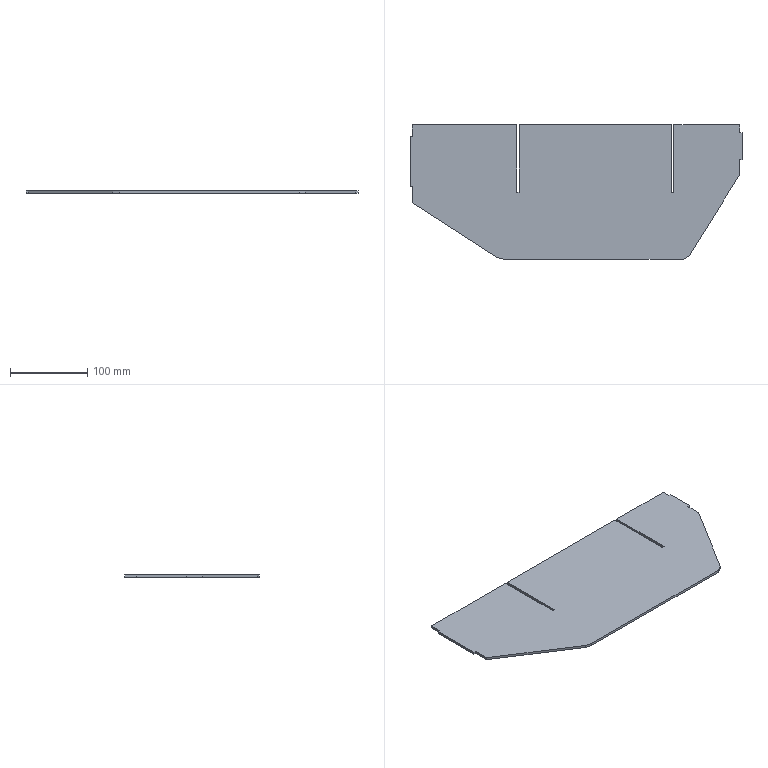Part | SolidWorks | features FlatPattern 1, SMBaseFlange 1, SheetMetal 1 | 1 solid | 26 faces | box 429 x 173.7 x 3.2 mm | volume 209173 mm3 | plane 26
STEP:
#1=CARTESIAN_POINT('',(256.891,49.63,0.));
#2=VERTEX_POINT('',#1);
#3=CARTESIAN_POINT('',(256.891,59.63,0.));
#4=VERTEX_POINT('',#3);
#5=CARTESIAN_POINT('',(256.891,59.63,0.));
#6=DIRECTION('',(0.,1.,0.));
#7=VECTOR('',#6,1000.);
#8=LINE('',#5,#7);
#9=EDGE_CURVE('',#2,#4,#8,.T.);
#10=ORIENTED_EDGE('',*,*,#9,.T.);
#11=CARTESIAN_POINT('',(256.891,59.63,3.2));
#12=VERTEX_POINT('',#11);
#13=CARTESIAN_POINT('',(256.891,59.63,3.2));
#14=DIRECTION('',(0.,0.,-1.));
#15=VECTOR('',#14,1000.);
#16=LINE('',#13,#15);
#17=EDGE_CURVE('',#12,#4,#16,.T.);
#18=ORIENTED_EDGE('',*,*,#17,.F.);
#19=CARTESIAN_POINT('',(256.891,49.63,3.2));
#20=VERTEX_POINT('',#19);
#21=CARTESIAN_POINT('',(256.891,59.63,3.2));
#22=DIRECTION('',(0.,1.,0.));
#23=VECTOR('',#22,1000.);
#24=LINE('',#21,#23);
#25=EDGE_CURVE('',#20,#12,#24,.T.);
#26=ORIENTED_EDGE('',*,*,#25,.F.);
#27=CARTESIAN_POINT('',(256.891,49.63,3.2));
#28=DIRECTION('',(0.,0.,-1.));
#29=VECTOR('',#28,1000.);
#30=LINE('',#27,#29);
#31=EDGE_CURVE('',#20,#2,#30,.T.);
#32=ORIENTED_EDGE('',*,*,#31,.T.);
#33=EDGE_LOOP('',(#10,#18,#26,#32));
#34=FACE_OUTER_BOUND('',#33,.T.);
#35=CARTESIAN_POINT('',(256.891,59.63,3.2));
#36=DIRECTION('',(-1.,0.,0.));
#37=DIRECTION('',(0.,0.,1.));
#38=AXIS2_PLACEMENT_3D('',#35,#36,#37);
#39=PLANE('',#38);
#40=ADVANCED_FACE('',(#34),#39,.F.);
#41=CARTESIAN_POINT('',(171.891,59.63,0.));
#42=VERTEX_POINT('',#41);
#43=CARTESIAN_POINT('',(256.891,59.63,0.));
#44=DIRECTION('',(-1.,0.,0.));
#45=VECTOR('',#44,1000.);
#46=LINE('',#43,#45);
#47=EDGE_CURVE('',#4,#42,#46,.T.);
#48=ORIENTED_EDGE('',*,*,#47,.T.);
#49=CARTESIAN_POINT('',(171.891,59.63,3.2));
#50=VERTEX_POINT('',#49);
#51=CARTESIAN_POINT('',(171.891,59.63,3.2));
#52=DIRECTION('',(0.,0.,-1.));
#53=VECTOR('',#52,1000.);
#54=LINE('',#51,#53);
#55=EDGE_CURVE('',#50,#42,#54,.T.);
#56=ORIENTED_EDGE('',*,*,#55,.F.);
#57=CARTESIAN_POINT('',(256.891,59.63,3.2));
#58=DIRECTION('',(-1.,0.,0.));
#59=VECTOR('',#58,1000.);
#60=LINE('',#57,#59);
#61=EDGE_CURVE('',#12,#50,#60,.T.);
#62=ORIENTED_EDGE('',*,*,#61,.F.);
#63=ORIENTED_EDGE('',*,*,#17,.T.);
#64=EDGE_LOOP('',(#48,#56,#62,#63));
#65=FACE_OUTER_BOUND('',#64,.T.);
#66=CARTESIAN_POINT('',(256.891,59.63,3.2));
#67=DIRECTION('',(0.,-1.,0.));
#68=DIRECTION('',(0.,0.,-1.));
#69=AXIS2_PLACEMENT_3D('',#66,#67,#68);
#70=PLANE('',#69);
#71=ADVANCED_FACE('',(#65),#70,.F.);
#72=CARTESIAN_POINT('',(171.891,-27.37,0.));
#73=VERTEX_POINT('',#72);
#74=CARTESIAN_POINT('',(171.891,-27.37,0.));
#75=DIRECTION('',(0.,-1.,0.));
#76=VECTOR('',#75,1000.);
#77=LINE('',#74,#76);
#78=EDGE_CURVE('',#42,#73,#77,.T.);
#79=ORIENTED_EDGE('',*,*,#78,.T.);
#80=CARTESIAN_POINT('',(171.891,-27.37,3.2));
#81=VERTEX_POINT('',#80);
#82=CARTESIAN_POINT('',(171.891,-27.37,3.2));
#83=DIRECTION('',(0.,0.,-1.));
#84=VECTOR('',#83,1000.);
#85=LINE('',#82,#84);
#86=EDGE_CURVE('',#81,#73,#85,.T.);
#87=ORIENTED_EDGE('',*,*,#86,.F.);
#88=CARTESIAN_POINT('',(171.891,-27.37,3.2));
#89=DIRECTION('',(0.,-1.,0.));
#90=VECTOR('',#89,1000.);
#91=LINE('',#88,#90);
#92=EDGE_CURVE('',#50,#81,#91,.T.);
#93=ORIENTED_EDGE('',*,*,#92,.F.);
#94=ORIENTED_EDGE('',*,*,#55,.T.);
#95=EDGE_LOOP('',(#79,#87,#93,#94));
#96=FACE_OUTER_BOUND('',#95,.T.);
#97=CARTESIAN_POINT('',(171.891,-27.37,3.2));
#98=DIRECTION('',(1.,0.,0.));
#99=DIRECTION('',(0.,1.,0.));
#100=AXIS2_PLACEMENT_3D('',#97,#98,#99);
#101=PLANE('',#100);
#102=ADVANCED_FACE('',(#96),#101,.F.);
#103=CARTESIAN_POINT('',(168.691,-27.37,0.));
#104=VERTEX_POINT('',#103);
#105=CARTESIAN_POINT('',(168.691,-27.37,0.));
#106=DIRECTION('',(-1.,0.,0.));
#107=VECTOR('',#106,1000.);
#108=LINE('',#105,#107);
#109=EDGE_CURVE('',#73,#104,#108,.T.);
#110=ORIENTED_EDGE('',*,*,#109,.T.);
#111=CARTESIAN_POINT('',(168.691,-27.37,3.2));
#112=VERTEX_POINT('',#111);
#113=CARTESIAN_POINT('',(168.691,-27.37,3.2));
#114=DIRECTION('',(0.,0.,-1.));
#115=VECTOR('',#114,1000.);
#116=LINE('',#113,#115);
#117=EDGE_CURVE('',#112,#104,#116,.T.);
#118=ORIENTED_EDGE('',*,*,#117,.F.);
#119=CARTESIAN_POINT('',(168.691,-27.37,3.2));
#120=DIRECTION('',(-1.,0.,0.));
#121=VECTOR('',#120,1000.);
#122=LINE('',#119,#121);
#123=EDGE_CURVE('',#81,#112,#122,.T.);
#124=ORIENTED_EDGE('',*,*,#123,.F.);
#125=ORIENTED_EDGE('',*,*,#86,.T.);
#126=EDGE_LOOP('',(#110,#118,#124,#125));
#127=FACE_OUTER_BOUND('',#126,.T.);
#128=CARTESIAN_POINT('',(168.691,-27.37,3.2));
#129=DIRECTION('',(0.,-1.,0.));
#130=DIRECTION('',(0.,0.,-1.));
#131=AXIS2_PLACEMENT_3D('',#128,#129,#130);
#132=PLANE('',#131);
#133=ADVANCED_FACE('',(#127),#132,.F.);
#134=CARTESIAN_POINT('',(168.691,59.63,0.));
#135=VERTEX_POINT('',#134);
#136=CARTESIAN_POINT('',(168.691,59.63,0.));
#137=DIRECTION('',(0.,1.,0.));
#138=VECTOR('',#137,1000.);
#139=LINE('',#136,#138);
#140=EDGE_CURVE('',#104,#135,#139,.T.);
#141=ORIENTED_EDGE('',*,*,#140,.T.);
#142=CARTESIAN_POINT('',(168.691,59.63,3.2));
#143=VERTEX_POINT('',#142);
#144=CARTESIAN_POINT('',(168.691,59.63,3.2));
#145=DIRECTION('',(0.,0.,-1.));
#146=VECTOR('',#145,1000.);
#147=LINE('',#144,#146);
#148=EDGE_CURVE('',#143,#135,#147,.T.);
#149=ORIENTED_EDGE('',*,*,#148,.F.);
#150=CARTESIAN_POINT('',(168.691,59.63,3.2));
#151=DIRECTION('',(0.,1.,0.));
#152=VECTOR('',#151,1000.);
#153=LINE('',#150,#152);
#154=EDGE_CURVE('',#112,#143,#153,.T.);
#155=ORIENTED_EDGE('',*,*,#154,.F.);
#156=ORIENTED_EDGE('',*,*,#117,.T.);
#157=EDGE_LOOP('',(#141,#149,#155,#156));
#158=FACE_OUTER_BOUND('',#157,.T.);
#159=CARTESIAN_POINT('',(168.691,59.63,3.2));
#160=DIRECTION('',(-1.,0.,0.));
#161=DIRECTION('',(0.,-1.,0.));
#162=AXIS2_PLACEMENT_3D('',#159,#160,#161);
#163=PLANE('',#162);
#164=ADVANCED_FACE('',(#158),#163,.F.);
#165=CARTESIAN_POINT('',(-28.109,59.63,0.));
#166=VERTEX_POINT('',#165);
#167=CARTESIAN_POINT('',(168.691,59.63,0.));
#168=DIRECTION('',(-1.,0.,0.));
#169=VECTOR('',#168,1000.);
#170=LINE('',#167,#169);
#171=EDGE_CURVE('',#135,#166,#170,.T.);
#172=ORIENTED_EDGE('',*,*,#171,.T.);
#173=CARTESIAN_POINT('',(-28.109,59.63,3.2));
#174=VERTEX_POINT('',#173);
#175=CARTESIAN_POINT('',(-28.109,59.63,3.2));
#176=DIRECTION('',(0.,0.,-1.));
#177=VECTOR('',#176,1000.);
#178=LINE('',#175,#177);
#179=EDGE_CURVE('',#174,#166,#178,.T.);
#180=ORIENTED_EDGE('',*,*,#179,.F.);
#181=CARTESIAN_POINT('',(168.691,59.63,3.2));
#182=DIRECTION('',(-1.,0.,0.));
#183=VECTOR('',#182,1000.);
#184=LINE('',#181,#183);
#185=EDGE_CURVE('',#143,#174,#184,.T.);
#186=ORIENTED_EDGE('',*,*,#185,.F.);
#187=ORIENTED_EDGE('',*,*,#148,.T.);
#188=EDGE_LOOP('',(#172,#180,#186,#187));
#189=FACE_OUTER_BOUND('',#188,.T.);
#190=CARTESIAN_POINT('',(168.691,59.63,3.2));
#191=DIRECTION('',(0.,-1.,0.));
#192=DIRECTION('',(0.,0.,-1.));
#193=AXIS2_PLACEMENT_3D('',#190,#191,#192);
#194=PLANE('',#193);
#195=ADVANCED_FACE('',(#189),#194,.F.);
#196=CARTESIAN_POINT('',(-28.109,-27.37,0.));
#197=VERTEX_POINT('',#196);
#198=CARTESIAN_POINT('',(-28.109,-27.37,0.));
#199=DIRECTION('',(0.,-1.,0.));
#200=VECTOR('',#199,1000.);
#201=LINE('',#198,#200);
#202=EDGE_CURVE('',#166,#197,#201,.T.);
#203=ORIENTED_EDGE('',*,*,#202,.T.);
#204=CARTESIAN_POINT('',(-28.109,-27.37,3.2));
#205=VERTEX_POINT('',#204);
#206=CARTESIAN_POINT('',(-28.109,-27.37,3.2));
#207=DIRECTION('',(0.,0.,-1.));
#208=VECTOR('',#207,1000.);
#209=LINE('',#206,#208);
#210=EDGE_CURVE('',#205,#197,#209,.T.);
#211=ORIENTED_EDGE('',*,*,#210,.F.);
#212=CARTESIAN_POINT('',(-28.109,-27.37,3.2));
#213=DIRECTION('',(0.,-1.,0.));
#214=VECTOR('',#213,1000.);
#215=LINE('',#212,#214);
#216=EDGE_CURVE('',#174,#205,#215,.T.);
#217=ORIENTED_EDGE('',*,*,#216,.F.);
#218=ORIENTED_EDGE('',*,*,#179,.T.);
#219=EDGE_LOOP('',(#203,#211,#217,#218));
#220=FACE_OUTER_BOUND('',#219,.T.);
#221=CARTESIAN_POINT('',(-28.109,-27.37,3.2));
#222=DIRECTION('',(1.,0.,0.));
#223=DIRECTION('',(0.,1.,0.));
#224=AXIS2_PLACEMENT_3D('',#221,#222,#223);
#225=PLANE('',#224);
#226=ADVANCED_FACE('',(#220),#225,.F.);
#227=CARTESIAN_POINT('',(-31.309,-27.37,0.));
#228=VERTEX_POINT('',#227);
#229=CARTESIAN_POINT('',(-31.309,-27.37,0.));
#230=DIRECTION('',(-1.,0.,0.));
#231=VECTOR('',#230,1000.);
#232=LINE('',#229,#231);
#233=EDGE_CURVE('',#197,#228,#232,.T.);
#234=ORIENTED_EDGE('',*,*,#233,.T.);
#235=CARTESIAN_POINT('',(-31.309,-27.37,3.2));
#236=VERTEX_POINT('',#235);
#237=CARTESIAN_POINT('',(-31.309,-27.37,3.2));
#238=DIRECTION('',(0.,0.,-1.));
#239=VECTOR('',#238,1000.);
#240=LINE('',#237,#239);
#241=EDGE_CURVE('',#236,#228,#240,.T.);
#242=ORIENTED_EDGE('',*,*,#241,.F.);
#243=CARTESIAN_POINT('',(-31.309,-27.37,3.2));
#244=DIRECTION('',(-1.,0.,0.));
#245=VECTOR('',#244,1000.);
#246=LINE('',#243,#245);
#247=EDGE_CURVE('',#205,#236,#246,.T.);
#248=ORIENTED_EDGE('',*,*,#247,.F.);
#249=ORIENTED_EDGE('',*,*,#210,.T.);
#250=EDGE_LOOP('',(#234,#242,#248,#249));
#251=FACE_OUTER_BOUND('',#250,.T.);
#252=CARTESIAN_POINT('',(-31.309,-27.37,3.2));
#253=DIRECTION('',(0.,-1.,0.));
#254=DIRECTION('',(0.,0.,-1.));
#255=AXIS2_PLACEMENT_3D('',#252,#253,#254);
#256=PLANE('',#255);
#257=ADVANCED_FACE('',(#251),#256,.F.);
#258=CARTESIAN_POINT('',(-31.309,59.63,0.));
#259=VERTEX_POINT('',#258);
#260=CARTESIAN_POINT('',(-31.309,59.63,0.));
#261=DIRECTION('',(0.,1.,0.));
#262=VECTOR('',#261,1000.);
#263=LINE('',#260,#262);
#264=EDGE_CURVE('',#228,#259,#263,.T.);
#265=ORIENTED_EDGE('',*,*,#264,.T.);
#266=CARTESIAN_POINT('',(-31.309,59.63,3.2));
#267=VERTEX_POINT('',#266);
#268=CARTESIAN_POINT('',(-31.309,59.63,3.2));
#269=DIRECTION('',(0.,0.,-1.));
#270=VECTOR('',#269,1000.);
#271=LINE('',#268,#270);
#272=EDGE_CURVE('',#267,#259,#271,.T.);
#273=ORIENTED_EDGE('',*,*,#272,.F.);
#274=CARTESIAN_POINT('',(-31.309,59.63,3.2));
#275=DIRECTION('',(0.,1.,0.));
#276=VECTOR('',#275,1000.);
#277=LINE('',#274,#276);
#278=EDGE_CURVE('',#236,#267,#277,.T.);
#279=ORIENTED_EDGE('',*,*,#278,.F.);
#280=ORIENTED_EDGE('',*,*,#241,.T.);
#281=EDGE_LOOP('',(#265,#273,#279,#280));
#282=FACE_OUTER_BOUND('',#281,.T.);
#283=CARTESIAN_POINT('',(-31.309,59.63,3.2));
#284=DIRECTION('',(-1.,0.,0.));
#285=DIRECTION('',(0.,-1.,0.));
#286=AXIS2_PLACEMENT_3D('',#283,#284,#285);
#287=PLANE('',#286);
#288=ADVANCED_FACE('',(#282),#287,.F.);
#289=CARTESIAN_POINT('',(-166.109,59.63,0.));
#290=VERTEX_POINT('',#289);
#291=CARTESIAN_POINT('',(-31.309,59.63,0.));
#292=DIRECTION('',(-1.,0.,0.));
#293=VECTOR('',#292,1000.);
#294=LINE('',#291,#293);
#295=EDGE_CURVE('',#259,#290,#294,.T.);
#296=ORIENTED_EDGE('',*,*,#295,.T.);
#297=CARTESIAN_POINT('',(-166.109,59.63,3.2));
#298=VERTEX_POINT('',#297);
#299=CARTESIAN_POINT('',(-166.109,59.63,3.2));
#300=DIRECTION('',(0.,0.,-1.));
#301=VECTOR('',#300,1000.);
#302=LINE('',#299,#301);
#303=EDGE_CURVE('',#298,#290,#302,.T.);
#304=ORIENTED_EDGE('',*,*,#303,.F.);
#305=CARTESIAN_POINT('',(-31.309,59.63,3.2));
#306=DIRECTION('',(-1.,0.,0.));
#307=VECTOR('',#306,1000.);
#308=LINE('',#305,#307);
#309=EDGE_CURVE('',#267,#298,#308,.T.);
#310=ORIENTED_EDGE('',*,*,#309,.F.);
#311=ORIENTED_EDGE('',*,*,#272,.T.);
#312=EDGE_LOOP('',(#296,#304,#310,#311));
#313=FACE_OUTER_BOUND('',#312,.T.);
#314=CARTESIAN_POINT('',(-31.309,59.63,3.2));
#315=DIRECTION('',(0.,-1.,0.));
#316=DIRECTION('',(0.,0.,-1.));
#317=AXIS2_PLACEMENT_3D('',#314,#315,#316);
#318=PLANE('',#317);
#319=ADVANCED_FACE('',(#313),#318,.F.);
#320=CARTESIAN_POINT('',(-166.109,44.63,0.));
#321=VERTEX_POINT('',#320);
#322=CARTESIAN_POINT('',(-166.109,59.63,0.));
#323=DIRECTION('',(0.,-1.,0.));
#324=VECTOR('',#323,1000.);
#325=LINE('',#322,#324);
#326=EDGE_CURVE('',#290,#321,#325,.T.);
#327=ORIENTED_EDGE('',*,*,#326,.T.);
#328=CARTESIAN_POINT('',(-166.109,44.63,3.2));
#329=VERTEX_POINT('',#328);
#330=CARTESIAN_POINT('',(-166.109,44.63,3.2));
#331=DIRECTION('',(0.,0.,-1.));
#332=VECTOR('',#331,1000.);
#333=LINE('',#330,#332);
#334=EDGE_CURVE('',#329,#321,#333,.T.);
#335=ORIENTED_EDGE('',*,*,#334,.F.);
#336=CARTESIAN_POINT('',(-166.109,59.63,3.2));
#337=DIRECTION('',(0.,-1.,0.));
#338=VECTOR('',#337,1000.);
#339=LINE('',#336,#338);
#340=EDGE_CURVE('',#298,#329,#339,.T.);
#341=ORIENTED_EDGE('',*,*,#340,.F.);
#342=ORIENTED_EDGE('',*,*,#303,.T.);
#343=EDGE_LOOP('',(#327,#335,#341,#342));
#344=FACE_OUTER_BOUND('',#343,.T.);
#345=CARTESIAN_POINT('',(-166.109,59.63,3.2));
#346=DIRECTION('',(1.,0.,0.));
#347=DIRECTION('',(0.,0.,-1.));
#348=AXIS2_PLACEMENT_3D('',#345,#346,#347);
#349=PLANE('',#348);
#350=ADVANCED_FACE('',(#344),#349,.F.);
#351=CARTESIAN_POINT('',(-169.109,44.63,0.));
#352=VERTEX_POINT('',#351);
#353=CARTESIAN_POINT('',(-169.109,44.63,0.));
#354=DIRECTION('',(-1.,0.,0.));
#355=VECTOR('',#354,1000.);
#356=LINE('',#353,#355);
#357=EDGE_CURVE('',#321,#352,#356,.T.);
#358=ORIENTED_EDGE('',*,*,#357,.T.);
#359=CARTESIAN_POINT('',(-169.109,44.63,3.2));
#360=VERTEX_POINT('',#359);
#361=CARTESIAN_POINT('',(-169.109,44.63,3.2));
#362=DIRECTION('',(0.,0.,-1.));
#363=VECTOR('',#362,1000.);
#364=LINE('',#361,#363);
#365=EDGE_CURVE('',#360,#352,#364,.T.);
#366=ORIENTED_EDGE('',*,*,#365,.F.);
#367=CARTESIAN_POINT('',(-169.109,44.63,3.2));
#368=DIRECTION('',(-1.,0.,0.));
#369=VECTOR('',#368,1000.);
#370=LINE('',#367,#369);
#371=EDGE_CURVE('',#329,#360,#370,.T.);
#372=ORIENTED_EDGE('',*,*,#371,.F.);
#373=ORIENTED_EDGE('',*,*,#334,.T.);
#374=EDGE_LOOP('',(#358,#366,#372,#373));
#375=FACE_OUTER_BOUND('',#374,.T.);
#376=CARTESIAN_POINT('',(-169.109,44.63,3.2));
#377=DIRECTION('',(0.,-1.,0.));
#378=DIRECTION('',(0.,0.,-1.));
#379=AXIS2_PLACEMENT_3D('',#376,#377,#378);
#380=PLANE('',#379);
#381=ADVANCED_FACE('',(#375),#380,.F.);
#382=CARTESIAN_POINT('',(-169.109,-20.37,0.));
#383=VERTEX_POINT('',#382);
#384=CARTESIAN_POINT('',(-169.109,-20.37,0.));
#385=DIRECTION('',(0.,-1.,0.));
#386=VECTOR('',#385,1000.);
#387=LINE('',#384,#386);
#388=EDGE_CURVE('',#352,#383,#387,.T.);
#389=ORIENTED_EDGE('',*,*,#388,.T.);
#390=CARTESIAN_POINT('',(-169.109,-20.37,3.2));
#391=VERTEX_POINT('',#390);
#392=CARTESIAN_POINT('',(-169.109,-20.37,3.2));
#393=DIRECTION('',(0.,0.,-1.));
#394=VECTOR('',#393,1000.);
#395=LINE('',#392,#394);
#396=EDGE_CURVE('',#391,#383,#395,.T.);
#397=ORIENTED_EDGE('',*,*,#396,.F.);
#398=CARTESIAN_POINT('',(-169.109,-20.37,3.2));
#399=DIRECTION('',(0.,-1.,0.));
#400=VECTOR('',#399,1000.);
#401=LINE('',#398,#400);
#402=EDGE_CURVE('',#360,#391,#401,.T.);
#403=ORIENTED_EDGE('',*,*,#402,.F.);
#404=ORIENTED_EDGE('',*,*,#365,.T.);
#405=EDGE_LOOP('',(#389,#397,#403,#404));
#406=FACE_OUTER_BOUND('',#405,.T.);
#407=CARTESIAN_POINT('',(-169.109,-20.37,3.2));
#408=DIRECTION('',(1.,0.,0.));
#409=DIRECTION('',(0.,0.,-1.));
#410=AXIS2_PLACEMENT_3D('',#407,#408,#409);
#411=PLANE('',#410);
#412=ADVANCED_FACE('',(#406),#411,.F.);
#413=CARTESIAN_POINT('',(-166.109,-20.37,0.));
#414=VERTEX_POINT('',#413);
#415=CARTESIAN_POINT('',(-166.109,-20.37,0.));
#416=DIRECTION('',(1.,0.,0.));
#417=VECTOR('',#416,1000.);
#418=LINE('',#415,#417);
#419=EDGE_CURVE('',#383,#414,#418,.T.);
#420=ORIENTED_EDGE('',*,*,#419,.T.);
#421=CARTESIAN_POINT('',(-166.109,-20.37,3.2));
#422=VERTEX_POINT('',#421);
#423=CARTESIAN_POINT('',(-166.109,-20.37,3.2));
#424=DIRECTION('',(0.,0.,-1.));
#425=VECTOR('',#424,1000.);
#426=LINE('',#423,#425);
#427=EDGE_CURVE('',#422,#414,#426,.T.);
#428=ORIENTED_EDGE('',*,*,#427,.F.);
#429=CARTESIAN_POINT('',(-166.109,-20.37,3.2));
#430=DIRECTION('',(1.,0.,0.));
#431=VECTOR('',#430,1000.);
#432=LINE('',#429,#431);
#433=EDGE_CURVE('',#391,#422,#432,.T.);
#434=ORIENTED_EDGE('',*,*,#433,.F.);
#435=ORIENTED_EDGE('',*,*,#396,.T.);
#436=EDGE_LOOP('',(#420,#428,#434,#435));
#437=FACE_OUTER_BOUND('',#436,.T.);
#438=CARTESIAN_POINT('',(-166.109,-20.37,3.2));
#439=DIRECTION('',(0.,1.,0.));
#440=DIRECTION('',(0.,0.,1.));
#441=AXIS2_PLACEMENT_3D('',#438,#439,#440);
#442=PLANE('',#441);
#443=ADVANCED_FACE('',(#437),#442,.F.);
#444=CARTESIAN_POINT('',(-166.109,-41.13,0.));
#445=VERTEX_POINT('',#444);
#446=CARTESIAN_POINT('',(-166.109,-20.37,0.));
#447=DIRECTION('',(0.,-1.,0.));
#448=VECTOR('',#447,1000.);
#449=LINE('',#446,#448);
#450=EDGE_CURVE('',#414,#445,#449,.T.);
#451=ORIENTED_EDGE('',*,*,#450,.T.);
#452=CARTESIAN_POINT('',(-166.109,-41.13,3.2));
#453=VERTEX_POINT('',#452);
#454=CARTESIAN_POINT('',(-166.109,-41.13,3.2));
#455=DIRECTION('',(0.,0.,-1.));
#456=VECTOR('',#455,1000.);
#457=LINE('',#454,#456);
#458=EDGE_CURVE('',#453,#445,#457,.T.);
#459=ORIENTED_EDGE('',*,*,#458,.F.);
#460=CARTESIAN_POINT('',(-166.109,-20.37,3.2));
#461=DIRECTION('',(0.,-1.,0.));
#462=VECTOR('',#461,1000.);
#463=LINE('',#460,#462);
#464=EDGE_CURVE('',#422,#453,#463,.T.);
#465=ORIENTED_EDGE('',*,*,#464,.F.);
#466=ORIENTED_EDGE('',*,*,#427,.T.);
#467=EDGE_LOOP('',(#451,#459,#465,#466));
#468=FACE_OUTER_BOUND('',#467,.T.);
#469=CARTESIAN_POINT('',(-166.109,-20.37,3.2));
#470=DIRECTION('',(1.,0.,0.));
#471=DIRECTION('',(0.,0.,-1.));
#472=AXIS2_PLACEMENT_3D('',#469,#470,#471);
#473=PLANE('',#472);
#474=ADVANCED_FACE('',(#468),#473,.F.);
#475=CARTESIAN_POINT('',(-56.877,-111.45,0.));
#476=VERTEX_POINT('',#475);
#477=CARTESIAN_POINT('',(-166.109,-41.13,0.));
#478=DIRECTION('',(0.8408,-0.5413,0.));
#479=VECTOR('',#478,1000.);
#480=LINE('',#477,#479);
#481=EDGE_CURVE('',#445,#476,#480,.T.);
#482=ORIENTED_EDGE('',*,*,#481,.T.);
#483=CARTESIAN_POINT('',(-56.877,-111.45,3.2));
#484=VERTEX_POINT('',#483);
#485=CARTESIAN_POINT('',(-56.877,-111.45,3.2));
#486=DIRECTION('',(0.,0.,-1.));
#487=VECTOR('',#486,1000.);
#488=LINE('',#485,#487);
#489=EDGE_CURVE('',#484,#476,#488,.T.);
#490=ORIENTED_EDGE('',*,*,#489,.F.);
#491=CARTESIAN_POINT('',(-166.109,-41.13,3.2));
#492=DIRECTION('',(0.8408,-0.5413,0.));
#493=VECTOR('',#492,1000.);
#494=LINE('',#491,#493);
#495=EDGE_CURVE('',#453,#484,#494,.T.);
#496=ORIENTED_EDGE('',*,*,#495,.F.);
#497=ORIENTED_EDGE('',*,*,#458,.T.);
#498=EDGE_LOOP('',(#482,#490,#496,#497));
#499=FACE_OUTER_BOUND('',#498,.T.);
#500=CARTESIAN_POINT('',(-166.109,-41.13,3.2));
#501=DIRECTION('',(0.5413,0.8408,0.));
#502=DIRECTION('',(-0.8408,0.5413,0.));
#503=AXIS2_PLACEMENT_3D('',#500,#501,#502);
#504=PLANE('',#503);
#505=ADVANCED_FACE('',(#499),#504,.F.);
#506=CARTESIAN_POINT('',(-47.809,-114.07,0.));
#507=VERTEX_POINT('',#506);
#508=CARTESIAN_POINT('',(-56.877,-111.45,0.));
#509=DIRECTION('',(0.9607,-0.2775,0.));
#510=VECTOR('',#509,1000.);
#511=LINE('',#508,#510);
#512=EDGE_CURVE('',#476,#507,#511,.T.);
#513=ORIENTED_EDGE('',*,*,#512,.T.);
#514=CARTESIAN_POINT('',(-47.809,-114.07,3.2));
#515=VERTEX_POINT('',#514);
#516=CARTESIAN_POINT('',(-47.809,-114.07,3.2));
#517=DIRECTION('',(0.,0.,-1.));
#518=VECTOR('',#517,1000.);
#519=LINE('',#516,#518);
#520=EDGE_CURVE('',#515,#507,#519,.T.);
#521=ORIENTED_EDGE('',*,*,#520,.F.);
#522=CARTESIAN_POINT('',(-56.877,-111.45,3.2));
#523=DIRECTION('',(0.9607,-0.2775,0.));
#524=VECTOR('',#523,1000.);
#525=LINE('',#522,#524);
#526=EDGE_CURVE('',#484,#515,#525,.T.);
#527=ORIENTED_EDGE('',*,*,#526,.F.);
#528=ORIENTED_EDGE('',*,*,#489,.T.);
#529=EDGE_LOOP('',(#513,#521,#527,#528));
#530=FACE_OUTER_BOUND('',#529,.T.);
#531=CARTESIAN_POINT('',(-56.877,-111.45,3.2));
#532=DIRECTION('',(0.2775,0.9607,0.));
#533=DIRECTION('',(-0.9607,0.2775,0.));
#534=AXIS2_PLACEMENT_3D('',#531,#532,#533);
#535=PLANE('',#534);
#536=ADVANCED_FACE('',(#530),#535,.F.);
#537=CARTESIAN_POINT('',(183.691,-114.07,0.));
#538=VERTEX_POINT('',#537);
#539=CARTESIAN_POINT('',(-47.809,-114.07,0.));
#540=DIRECTION('',(1.,0.,0.));
#541=VECTOR('',#540,1000.);
#542=LINE('',#539,#541);
#543=EDGE_CURVE('',#507,#538,#542,.T.);
#544=ORIENTED_EDGE('',*,*,#543,.T.);
#545=CARTESIAN_POINT('',(183.691,-114.07,3.2));
#546=VERTEX_POINT('',#545);
#547=CARTESIAN_POINT('',(183.691,-114.07,3.2));
#548=DIRECTION('',(0.,0.,-1.));
#549=VECTOR('',#548,1000.);
#550=LINE('',#547,#549);
#551=EDGE_CURVE('',#546,#538,#550,.T.);
#552=ORIENTED_EDGE('',*,*,#551,.F.);
#553=CARTESIAN_POINT('',(-47.809,-114.07,3.2));
#554=DIRECTION('',(1.,0.,0.));
#555=VECTOR('',#554,1000.);
#556=LINE('',#553,#555);
#557=EDGE_CURVE('',#515,#546,#556,.T.);
#558=ORIENTED_EDGE('',*,*,#557,.F.);
#559=ORIENTED_EDGE('',*,*,#520,.T.);
#560=EDGE_LOOP('',(#544,#552,#558,#559));
#561=FACE_OUTER_BOUND('',#560,.T.);
#562=CARTESIAN_POINT('',(-47.809,-114.07,3.2));
#563=DIRECTION('',(0.,1.,0.));
#564=DIRECTION('',(-1.,0.,0.));
#565=AXIS2_PLACEMENT_3D('',#562,#563,#564);
#566=PLANE('',#565);
#567=ADVANCED_FACE('',(#561),#566,.F.);
#568=CARTESIAN_POINT('',(191.955,-109.489,0.));
#569=VERTEX_POINT('',#568);
#570=CARTESIAN_POINT('',(183.691,-114.07,0.));
#571=DIRECTION('',(0.8746,0.4848,0.));
#572=VECTOR('',#571,1000.);
#573=LINE('',#570,#572);
#574=EDGE_CURVE('',#538,#569,#573,.T.);
#575=ORIENTED_EDGE('',*,*,#574,.T.);
#576=CARTESIAN_POINT('',(191.955,-109.489,3.2));
#577=VERTEX_POINT('',#576);
#578=CARTESIAN_POINT('',(191.955,-109.489,3.2));
#579=DIRECTION('',(0.,0.,-1.));
#580=VECTOR('',#579,1000.);
#581=LINE('',#578,#580);
#582=EDGE_CURVE('',#577,#569,#581,.T.);
#583=ORIENTED_EDGE('',*,*,#582,.F.);
#584=CARTESIAN_POINT('',(183.691,-114.07,3.2));
#585=DIRECTION('',(0.8746,0.4848,0.));
#586=VECTOR('',#585,1000.);
#587=LINE('',#584,#586);
#588=EDGE_CURVE('',#546,#577,#587,.T.);
#589=ORIENTED_EDGE('',*,*,#588,.F.);
#590=ORIENTED_EDGE('',*,*,#551,.T.);
#591=EDGE_LOOP('',(#575,#583,#589,#590));
#592=FACE_OUTER_BOUND('',#591,.T.);
#593=CARTESIAN_POINT('',(183.691,-114.07,3.2));
#594=DIRECTION('',(-0.4848,0.8746,0.));
#595=DIRECTION('',(-0.8746,-0.4848,0.));
#596=AXIS2_PLACEMENT_3D('',#593,#594,#595);
#597=PLANE('',#596);
#598=ADVANCED_FACE('',(#592),#597,.F.);
#599=CARTESIAN_POINT('',(256.891,-4.869,0.));
#600=VERTEX_POINT('',#599);
#601=CARTESIAN_POINT('',(191.955,-109.489,0.));
#602=DIRECTION('',(0.5274,0.8496,0.));
#603=VECTOR('',#602,1000.);
#604=LINE('',#601,#603);
#605=EDGE_CURVE('',#569,#600,#604,.T.);
#606=ORIENTED_EDGE('',*,*,#605,.T.);
#607=CARTESIAN_POINT('',(256.891,-4.869,3.2));
#608=VERTEX_POINT('',#607);
#609=CARTESIAN_POINT('',(256.891,-4.869,3.2));
#610=DIRECTION('',(0.,0.,-1.));
#611=VECTOR('',#610,1000.);
#612=LINE('',#609,#611);
#613=EDGE_CURVE('',#608,#600,#612,.T.);
#614=ORIENTED_EDGE('',*,*,#613,.F.);
#615=CARTESIAN_POINT('',(191.955,-109.489,3.2));
#616=DIRECTION('',(0.5274,0.8496,0.));
#617=VECTOR('',#616,1000.);
#618=LINE('',#615,#617);
#619=EDGE_CURVE('',#577,#608,#618,.T.);
#620=ORIENTED_EDGE('',*,*,#619,.F.);
#621=ORIENTED_EDGE('',*,*,#582,.T.);
#622=EDGE_LOOP('',(#606,#614,#620,#621));
#623=FACE_OUTER_BOUND('',#622,.T.);
#624=CARTESIAN_POINT('',(191.955,-109.489,3.2));
#625=DIRECTION('',(-0.8496,0.5274,0.));
#626=DIRECTION('',(-0.5274,-0.8496,0.));
#627=AXIS2_PLACEMENT_3D('',#624,#625,#626);
#628=PLANE('',#627);
#629=ADVANCED_FACE('',(#623),#628,.F.);
#630=CARTESIAN_POINT('',(256.891,14.63,0.));
#631=VERTEX_POINT('',#630);
#632=CARTESIAN_POINT('',(256.891,14.63,0.));
#633=DIRECTION('',(0.,1.,0.));
#634=VECTOR('',#633,1000.);
#635=LINE('',#632,#634);
#636=EDGE_CURVE('',#600,#631,#635,.T.);
#637=ORIENTED_EDGE('',*,*,#636,.T.);
#638=CARTESIAN_POINT('',(256.891,14.63,3.2));
#639=VERTEX_POINT('',#638);
#640=CARTESIAN_POINT('',(256.891,14.63,3.2));
#641=DIRECTION('',(0.,0.,-1.));
#642=VECTOR('',#641,1000.);
#643=LINE('',#640,#642);
#644=EDGE_CURVE('',#639,#631,#643,.T.);
#645=ORIENTED_EDGE('',*,*,#644,.F.);
#646=CARTESIAN_POINT('',(256.891,14.63,3.2));
#647=DIRECTION('',(0.,1.,0.));
#648=VECTOR('',#647,1000.);
#649=LINE('',#646,#648);
#650=EDGE_CURVE('',#608,#639,#649,.T.);
#651=ORIENTED_EDGE('',*,*,#650,.F.);
#652=ORIENTED_EDGE('',*,*,#613,.T.);
#653=EDGE_LOOP('',(#637,#645,#651,#652));
#654=FACE_OUTER_BOUND('',#653,.T.);
#655=CARTESIAN_POINT('',(256.891,14.63,3.2));
#656=DIRECTION('',(-1.,0.,0.));
#657=DIRECTION('',(0.,0.,1.));
#658=AXIS2_PLACEMENT_3D('',#655,#656,#657);
#659=PLANE('',#658);
#660=ADVANCED_FACE('',(#654),#659,.F.);
#661=CARTESIAN_POINT('',(259.891,14.63,0.));
#662=VERTEX_POINT('',#661);
#663=CARTESIAN_POINT('',(256.891,14.63,0.));
#664=DIRECTION('',(1.,0.,0.));
#665=VECTOR('',#664,1000.);
#666=LINE('',#663,#665);
#667=EDGE_CURVE('',#631,#662,#666,.T.);
#668=ORIENTED_EDGE('',*,*,#667,.T.);
#669=CARTESIAN_POINT('',(259.891,14.63,3.2));
#670=VERTEX_POINT('',#669);
#671=CARTESIAN_POINT('',(259.891,14.63,3.2));
#672=DIRECTION('',(0.,0.,-1.));
#673=VECTOR('',#672,1000.);
#674=LINE('',#671,#673);
#675=EDGE_CURVE('',#670,#662,#674,.T.);
#676=ORIENTED_EDGE('',*,*,#675,.F.);
#677=CARTESIAN_POINT('',(256.891,14.63,3.2));
#678=DIRECTION('',(1.,0.,0.));
#679=VECTOR('',#678,1000.);
#680=LINE('',#677,#679);
#681=EDGE_CURVE('',#639,#670,#680,.T.);
#682=ORIENTED_EDGE('',*,*,#681,.F.);
#683=ORIENTED_EDGE('',*,*,#644,.T.);
#684=EDGE_LOOP('',(#668,#676,#682,#683));
#685=FACE_OUTER_BOUND('',#684,.T.);
#686=CARTESIAN_POINT('',(256.891,14.63,3.2));
#687=DIRECTION('',(0.,1.,0.));
#688=DIRECTION('',(0.,0.,1.));
#689=AXIS2_PLACEMENT_3D('',#686,#687,#688);
#690=PLANE('',#689);
#691=ADVANCED_FACE('',(#685),#690,.F.);
#692=CARTESIAN_POINT('',(259.891,49.63,0.));
#693=VERTEX_POINT('',#692);
#694=CARTESIAN_POINT('',(259.891,14.63,0.));
#695=DIRECTION('',(0.,1.,0.));
#696=VECTOR('',#695,1000.);
#697=LINE('',#694,#696);
#698=EDGE_CURVE('',#662,#693,#697,.T.);
#699=ORIENTED_EDGE('',*,*,#698,.T.);
#700=CARTESIAN_POINT('',(259.891,49.63,3.2));
#701=VERTEX_POINT('',#700);
#702=CARTESIAN_POINT('',(259.891,49.63,3.2));
#703=DIRECTION('',(0.,0.,-1.));
#704=VECTOR('',#703,1000.);
#705=LINE('',#702,#704);
#706=EDGE_CURVE('',#701,#693,#705,.T.);
#707=ORIENTED_EDGE('',*,*,#706,.F.);
#708=CARTESIAN_POINT('',(259.891,14.63,3.2));
#709=DIRECTION('',(0.,1.,0.));
#710=VECTOR('',#709,1000.);
#711=LINE('',#708,#710);
#712=EDGE_CURVE('',#670,#701,#711,.T.);
#713=ORIENTED_EDGE('',*,*,#712,.F.);
#714=ORIENTED_EDGE('',*,*,#675,.T.);
#715=EDGE_LOOP('',(#699,#707,#713,#714));
#716=FACE_OUTER_BOUND('',#715,.T.);
#717=CARTESIAN_POINT('',(259.891,14.63,3.2));
#718=DIRECTION('',(-1.,0.,0.));
#719=DIRECTION('',(0.,0.,1.));
#720=AXIS2_PLACEMENT_3D('',#717,#718,#719);
#721=PLANE('',#720);
#722=ADVANCED_FACE('',(#716),#721,.F.);
#723=CARTESIAN_POINT('',(259.891,49.63,0.));
#724=DIRECTION('',(-1.,0.,0.));
#725=VECTOR('',#724,1000.);
#726=LINE('',#723,#725);
#727=EDGE_CURVE('',#693,#2,#726,.T.);
#728=ORIENTED_EDGE('',*,*,#727,.T.);
#729=ORIENTED_EDGE('',*,*,#31,.F.);
#730=CARTESIAN_POINT('',(259.891,49.63,3.2));
#731=DIRECTION('',(-1.,0.,0.));
#732=VECTOR('',#731,1000.);
#733=LINE('',#730,#732);
#734=EDGE_CURVE('',#701,#20,#733,.T.);
#735=ORIENTED_EDGE('',*,*,#734,.F.);
#736=ORIENTED_EDGE('',*,*,#706,.T.);
#737=EDGE_LOOP('',(#728,#729,#735,#736));
#738=FACE_OUTER_BOUND('',#737,.T.);
#739=CARTESIAN_POINT('',(259.891,49.63,3.2));
#740=DIRECTION('',(0.,-1.,0.));
#741=DIRECTION('',(0.,0.,-1.));
#742=AXIS2_PLACEMENT_3D('',#739,#740,#741);
#743=PLANE('',#742);
#744=ADVANCED_FACE('',(#738),#743,.F.);
#745=ORIENTED_EDGE('',*,*,#25,.T.);
#746=ORIENTED_EDGE('',*,*,#61,.T.);
#747=ORIENTED_EDGE('',*,*,#92,.T.);
#748=ORIENTED_EDGE('',*,*,#123,.T.);
#749=ORIENTED_EDGE('',*,*,#154,.T.);
#750=ORIENTED_EDGE('',*,*,#185,.T.);
#751=ORIENTED_EDGE('',*,*,#216,.T.);
#752=ORIENTED_EDGE('',*,*,#247,.T.);
#753=ORIENTED_EDGE('',*,*,#278,.T.);
#754=ORIENTED_EDGE('',*,*,#309,.T.);
#755=ORIENTED_EDGE('',*,*,#340,.T.);
#756=ORIENTED_EDGE('',*,*,#371,.T.);
#757=ORIENTED_EDGE('',*,*,#402,.T.);
#758=ORIENTED_EDGE('',*,*,#433,.T.);
#759=ORIENTED_EDGE('',*,*,#464,.T.);
#760=ORIENTED_EDGE('',*,*,#495,.T.);
#761=ORIENTED_EDGE('',*,*,#526,.T.);
#762=ORIENTED_EDGE('',*,*,#557,.T.);
#763=ORIENTED_EDGE('',*,*,#588,.T.);
#764=ORIENTED_EDGE('',*,*,#619,.T.);
#765=ORIENTED_EDGE('',*,*,#650,.T.);
#766=ORIENTED_EDGE('',*,*,#681,.T.);
#767=ORIENTED_EDGE('',*,*,#712,.T.);
#768=ORIENTED_EDGE('',*,*,#734,.T.);
#769=EDGE_LOOP('',(#745,#746,#747,#748,#749,#750,#751,#752,#753,#754,#755,#756,#757,#758,#759,#760,#761,#762,#763,#764,#765,#766,#767,#768));
#770=FACE_OUTER_BOUND('',#769,.T.);
#771=CARTESIAN_POINT('',(0.,0.,3.2));
#772=DIRECTION('',(0.,0.,-1.));
#773=DIRECTION('',(-1.,0.,0.));
#774=AXIS2_PLACEMENT_3D('',#771,#772,#773);
#775=PLANE('',#774);
#776=ADVANCED_FACE('',(#770),#775,.F.);
#777=ORIENTED_EDGE('',*,*,#9,.F.);
#778=ORIENTED_EDGE('',*,*,#727,.F.);
#779=ORIENTED_EDGE('',*,*,#698,.F.);
#780=ORIENTED_EDGE('',*,*,#667,.F.);
#781=ORIENTED_EDGE('',*,*,#636,.F.);
#782=ORIENTED_EDGE('',*,*,#605,.F.);
#783=ORIENTED_EDGE('',*,*,#574,.F.);
#784=ORIENTED_EDGE('',*,*,#543,.F.);
#785=ORIENTED_EDGE('',*,*,#512,.F.);
#786=ORIENTED_EDGE('',*,*,#481,.F.);
#787=ORIENTED_EDGE('',*,*,#450,.F.);
#788=ORIENTED_EDGE('',*,*,#419,.F.);
#789=ORIENTED_EDGE('',*,*,#388,.F.);
#790=ORIENTED_EDGE('',*,*,#357,.F.);
#791=ORIENTED_EDGE('',*,*,#326,.F.);
#792=ORIENTED_EDGE('',*,*,#295,.F.);
#793=ORIENTED_EDGE('',*,*,#264,.F.);
#794=ORIENTED_EDGE('',*,*,#233,.F.);
#795=ORIENTED_EDGE('',*,*,#202,.F.);
#796=ORIENTED_EDGE('',*,*,#171,.F.);
#797=ORIENTED_EDGE('',*,*,#140,.F.);
#798=ORIENTED_EDGE('',*,*,#109,.F.);
#799=ORIENTED_EDGE('',*,*,#78,.F.);
#800=ORIENTED_EDGE('',*,*,#47,.F.);
#801=EDGE_LOOP('',(#777,#778,#779,#780,#781,#782,#783,#784,#785,#786,#787,#788,#789,#790,#791,#792,#793,#794,#795,#796,#797,#798,#799,#800));
#802=FACE_OUTER_BOUND('',#801,.T.);
#803=CARTESIAN_POINT('',(0.,0.,0.));
#804=DIRECTION('',(0.,0.,-1.));
#805=DIRECTION('',(-1.,0.,0.));
#806=AXIS2_PLACEMENT_3D('',#803,#804,#805);
#807=PLANE('',#806);
#808=ADVANCED_FACE('',(#802),#807,.T.);
#809=CLOSED_SHELL('',(#40,#71,#102,#133,#164,#195,#226,#257,#288,#319,#350,#381,#412,#443,#474,#505,#536,#567,#598,#629,#660,#691,#722,#744,#776,#808));
#810=MANIFOLD_SOLID_BREP('',#809);
#811=CARTESIAN_POINT('',(0.,0.,0.));
#812=DIRECTION('',(0.,0.,1.));
#813=DIRECTION('',(1.,0.,0.));
#814=AXIS2_PLACEMENT_3D('',#811,#812,#813);
#815=(LENGTH_UNIT()NAMED_UNIT(*)SI_UNIT(.MILLI.,.METRE.));
#816=UNCERTAINTY_MEASURE_WITH_UNIT(LENGTH_MEASURE(0.00001),#815,'','');
#817=(NAMED_UNIT(*)PLANE_ANGLE_UNIT()SI_UNIT($,.RADIAN.));
#818=(NAMED_UNIT(*)SI_UNIT($,.STERADIAN.)SOLID_ANGLE_UNIT());
#819=(GEOMETRIC_REPRESENTATION_CONTEXT(3)GLOBAL_UNCERTAINTY_ASSIGNED_CONTEXT((#816))GLOBAL_UNIT_ASSIGNED_CONTEXT((#815,#817,#818))REPRESENTATION_CONTEXT('',''));
#820=ADVANCED_BREP_SHAPE_REPRESENTATION('',(#810,#814),#819);